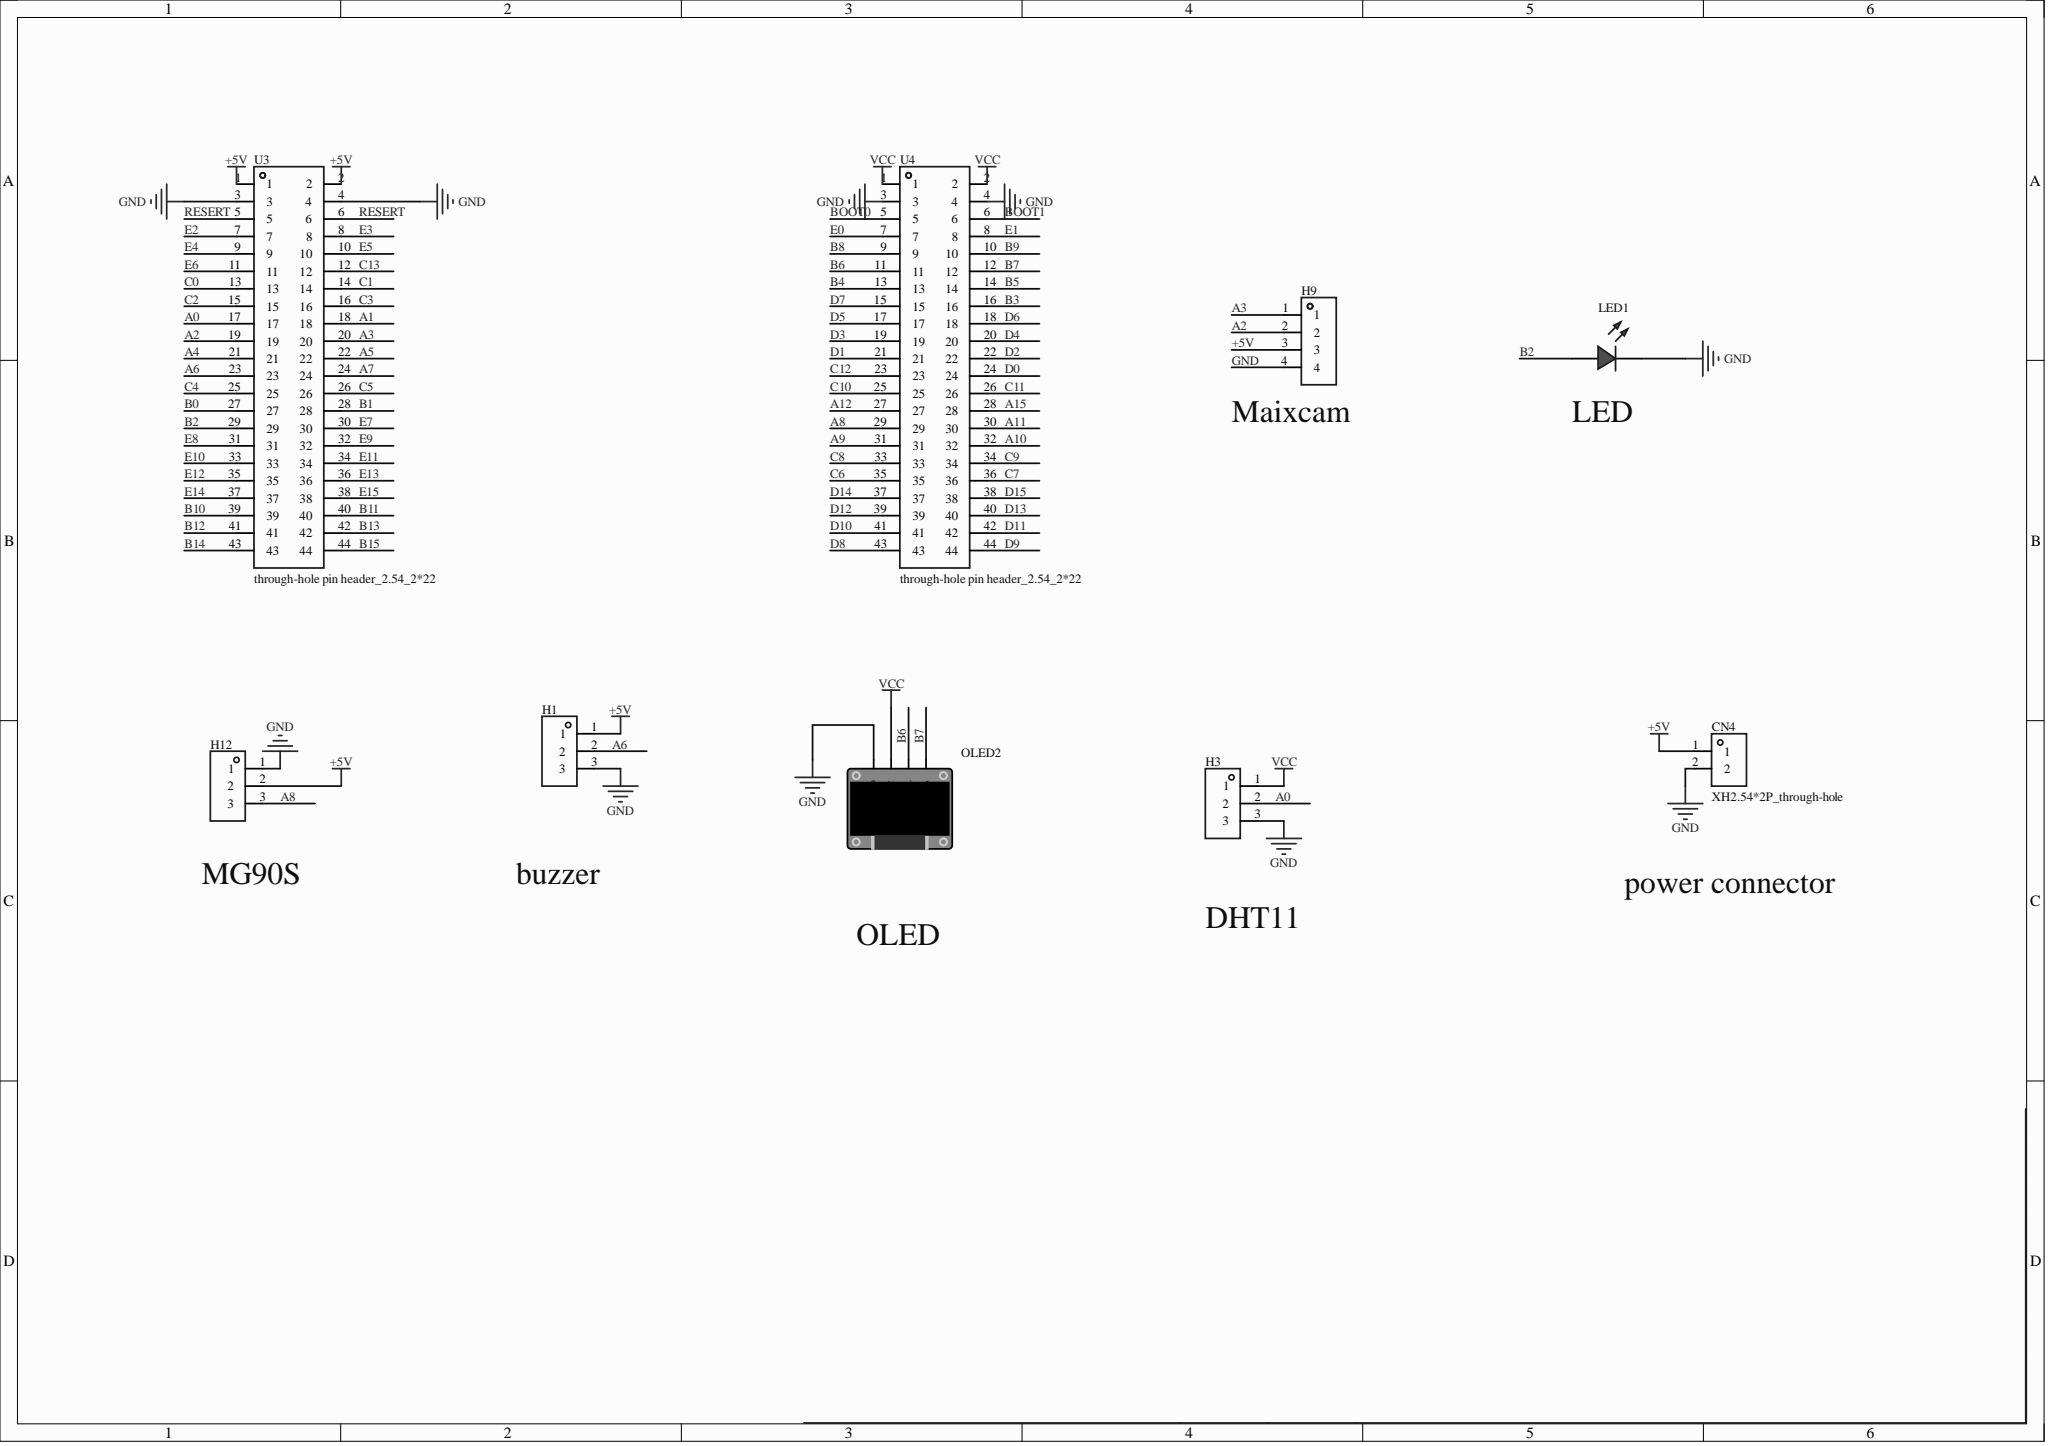Circuit board | Altium Designer | 9 parts | 12 nets
Bill of materials:
Comment,Description,Designator,Footprint,LibRef,Quantity
"XH2.54*2P_through-hole","","CN4","CONN-TH_2P-P2.50-XH2.54-2P","XH2.54*2P_直插","1"
"","","H1, H3, H12","HDR-TH_3P-P2.54-V-F","HDR-F_2.54_1x3P","3"
"","","H9","HDR-TH_4P-P2.54-V-F","HDR-F_2.54_1x4P","1"
"","","LED1","LED_TH-3mm","LED_TH-R_3mm","1"
"","","OLED2","0.96OLED_4P","0.96OLED模块_4P","1"
"through-hole pin header_2.54_2*22","","U3, U4","HDR-TH_44P-P2.54-V-M-R2-C22-S2.54","直插排针_2.54_2*22","2"
Netlist (Protel format):
[
CN4
CONN-TH_2P-P2.50-XH2.54-2P
XH2.54*2P_through-hole



]
[
H1
HDR-TH_3P-P2.54-V-F




]
[
H3
HDR-TH_3P-P2.54-V-F




]
[
H9
HDR-TH_4P-P2.54-V-F




]
[
H12
HDR-TH_3P-P2.54-V-F




]
[
LED1
LED_TH-3mm




]
[
OLED2
0.96OLED_4P




]
[
U3
HDR-TH_44P-P2.54-V-M-R2-C22-S2.54
through-hole pin header_2.54_2*22



]
[
U4
HDR-TH_44P-P2.54-V-M-R2-C22-S2.54
through-hole pin header_2.54_2*22



]
(
VCC
H3-1
OLED2-2
U4-1
U4-2
)
(
RESERT
U3-5
U3-6
)
(
GND
CN4-2
H1-3
H3-3
H9-4
H12-1
LED1-2
OLED2-1
U3-3
U3-4
U4-3
U4-4
)
(
B7
OLED2-4
U4-12
)
(
B6
OLED2-3
U4-11
)
(
B2
LED1-1
U3-29
)
(
A8
H12-3
U4-29
)
(
A6
H1-2
U3-23
)
(
A3
H9-1
U3-20
)
(
A2
H9-2
U3-19
)
(
A0
H3-2
U3-17
)
(
+5V
CN4-1
H1-1
H9-3
H12-2
U3-1
U3-2
)